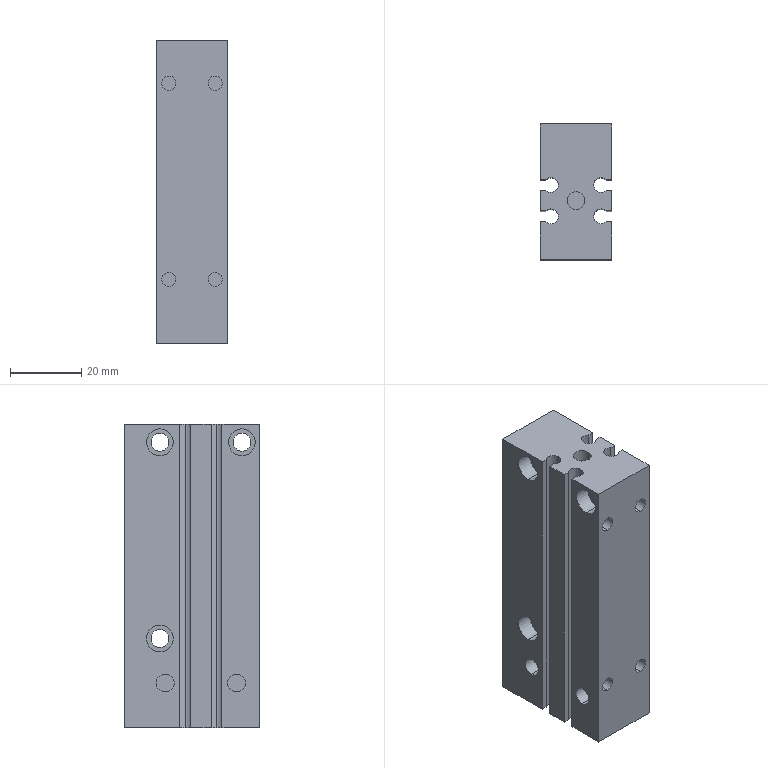Part | NX | 1 solid | 96 faces | box 20 x 38 x 85 mm | volume 51301 mm3 | cylinder 56 | plane 40 | commonest cylinder face diameters 5 x20 4 x16 7.5 x12 4.15 x6 10 x2